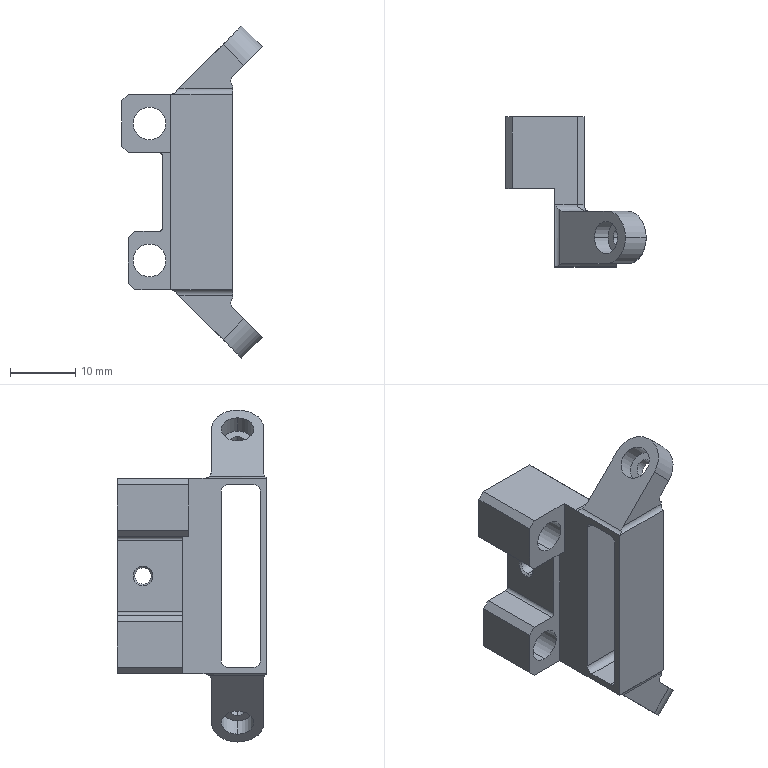NC program | NX | posted with a generic post | part box 21.534 x 23 x 50.912 mm
Lines 1 to 848 of 6474:
N10 G17 G21 G94 G90
(FLOOR_FACING , TOOL : D8开粗)
N12 T01 M6
N14 G54
N16 G17 G0 G90 X35. Y-12.5 B0. C0. S1061 M3
N18 G43 Z53. H1
N20 Z3.1
N22 G94 G1 Z0.1 F250.
N24 X34.
N26 G3 X32. Y-10.5 R2.
N28 G1 X-32.
N30 Y-5.55
N32 X32.
N34 Y-0.6
N36 X-32.
N38 Y4.35
N40 X32.
N42 Y9.3
N44 X-32.
N46 G3 X-34. Y7.3 R2.
N48 G1 X-35.
N50 Z3.1
N52 G0 Z53.
(ADAPTIVE_MILLING , TOOL : D8开粗)
N54 X37.12 Y1.02
N56 Z50.15
N58 Z-8.75
N60 G1 X36.97 Y1.008 Z-9.687
N62 X36.821 Y0.996 Z-10.058
N64 X36.671 Y0.985 Z-10.33
N66 X36.522 Y0.973 Z-10.55
N68 X36.372 Y0.961 Z-10.734
N70 X36.223 Y0.949 Z-10.892
N72 X36.073 Y0.938 Z-11.03
N74 X35.924 Y0.926 Z-11.15
N76 X35.774 Y0.914 Z-11.255
N78 X35.625 Y0.903 Z-11.348
N80 X35.475 Y0.891 Z-11.429
N82 X35.325 Y0.879 Z-11.5
N84 X35.176 Y0.867 Z-11.56
N86 X35.026 Y0.856 Z-11.612
N88 X34.877 Y0.844 Z-11.655
N90 X34.727 Y0.832 Z-11.689
N92 X34.578 Y0.821 Z-11.716
N94 X34.428 Y0.809 Z-11.735
N96 X34.279 Y0.797 Z-11.746
N98 X34.129 Y0.785 Z-11.75
N100 X32.743 Y0.677
N102 G3 X32.087 Y0.238 R0.809
N104 X31.465 Y-2.339 R7.41
N106 X31.241 Y-8.744 R74.09
N108 G2 X31.185 Y-10.771 R16.326
N110 X29.104 Y-13.79 R4.795
N112 X25.181 Y-15.269 R9.684
N114 X19.381 Y-15.687 R39.045
N116 X9.602 Y-15.727 R696.065
N118 G1 X-25.793 Y-15.726
N120 G2 X-28.856 Y-14.155 R4.335
N122 X-30.639 Y-10.333 R8.413
N124 X-31.16 Y-4.966 R29.566
N126 X-31.212 Y10.529 R651.721
N128 X-29.4 Y13.594 R4.522
N130 X-25.566 Y15.208 R8.891
N132 X-20.012 Y15.675 R33.85
N134 X-9.272 Y15.728 R699.457
N136 G1 X25.841 Y15.725
N138 G2 X29.013 Y14.001 R4.415
N140 X30.693 Y10.133 R8.704
N142 X31.174 Y4.52 R33.321
N144 X30.916 Y-0.16 R24.978
N146 G3 X30.457 Y-8.115 R78.765
N148 G2 X27.712 Y-12.707 R6.046
N150 X23.193 Y-14.403 R11.375
N152 X16.917 Y-14.876 R41.945
N154 X4.087 Y-14.924 R878.762
N156 G1 X-0.233 Y-14.927
N158 X-23.406 Y-14.925
N160 G2 X-28.115 Y-12.318 R5.94
N162 X-29.863 Y-7.885 R10.966
N164 X-30.367 Y-1.792 R38.718
N166 X-30.407 Y8.287 R314.055
N168 X-27.773 Y12.664 R5.962
N170 X-23.265 Y14.392 R11.16
N172 X-17.11 Y14.874 R40.717
N174 X-6.55 Y14.927 R694.796
N176 G1 X23.44 Y14.925
N178 G2 X28.138 Y12.306 R5.921
N180 X29.884 Y7.805 R11.093
N182 X30.132 Y0.751 R26.451
N184 G3 X29.694 Y-6.493 R229.838
N186 G2 X26.24 Y-11.917 R7.083
N188 X21.328 Y-13.608 R13.219
N190 X16.67 Y-14.034 R47.013
N192 G3 X16.304 Y-14.218 R1.352
N194 G2 X14.032 Y-14.914 R4.432
N196 G3 X16.495 Y-14.066 R4.204
N198 G2 X18.579 Y-13.556 R8.285
N200 G3 X23.029 Y-12.653 R30.768
N202 X27.011 Y-10.273 R8.809
N204 X28.853 Y-6.398 R8.238
N206 X29.458 Y-1.579 R39.94
N208 X29.703 Y4.352 R45.756
N210 X28.814 Y9.475 R17.252
N212 X26.213 Y12.898 R6.567
N214 X22.308 Y14.169 R9.553
N216 X16.977 Y14.431 R46.853
N218 G1 X10.977 Y14.447
N220 X-10.063 Y14.445
N222 G3 X-19.6 Y14.277 R171.741
N224 X-24.618 Y13.448 R20.333
N226 X-27.927 Y11.363 R7.158
N228 X-29.544 Y7.594 R8.07
N230 X-29.906 Y2.453 R31.43
N232 X-29.622 Y-5.818 R72.414
N234 X-28.473 Y-10.271 R13.972
N236 X-24.269 Y-13.763 R6.431
N238 X-19.941 Y-14.362 R18.143
N240 X-9.142 Y-14.447 R324.916
N242 G1 X3.318 Y-14.445
N244 G2 X5.099 Y-14.465 R18.722
N246 G3 X6.999 Y-14.917 R4.927
N248 G2 X4.896 Y-14.335 R4.42
N250 G3 X1.969 Y-13.818 R10.606
N252 X-5.593 Y-13.663 R111.649
N254 G2 X-7.001 Y-13.917 R4.701
N256 G1 X-14.001
N258 G3 X-19.53 Y-13.568 R111.918
N260 G2 X-23.365 Y-12.927 R14.578
N262 X-27.379 Y-9.236 R7.304
N264 X-28.751 Y-4.343 R14.883
N266 X-28.898 Y5.599 R49.455
N268 X-27.819 Y9.127 R8.415
N270 X-24.01 Y12.22 R7.937
N272 X-18.872 Y13.364 R17.751
N274 X-10.479 Y13.637 R99.34
N276 G1 X-3.639 Y13.647
N278 X12.961 Y13.645
N280 G2 X20.337 Y13.487 R104.564
N282 X23.841 Y12.733 R10.991
N284 X27.503 Y8.968 R7.427
N286 X28.724 Y3.434 R14.681
N288 X28.181 Y-5.054 R41.969
N290 X23.713 Y-10.998 R8.122
N292 X19.632 Y-12.405 R18.072
N294 G3 X17.794 Y-12.905 R28.33
N296 G1 X17.601 Y-13.035
N298 G2 X16.424 Y-14.12 R9.618
N300 G3 X17.729 Y-12.908 R10.801
N302 G2 X19.648 Y-12.042 R7.886
N304 G3 X23.329 Y-10.5 R20.797
N306 X27.297 Y-5.403 R8.58
N308 X28.174 Y0.275 R23.637
N310 X27.748 Y6.299 R20.911
N312 X25.598 Y10.397 R8.618
N314 X21.373 Y12.578 R8.611
N316 X16.129 Y13.11 R27.016
N318 X7.189 Y13.166 R509.255
N320 G1 X-7.191 Y13.164
N322 G3 X-17.268 Y12.979 R172.599
N324 X-22.634 Y12.06 R21.257
N326 X-26.611 Y9.275 R7.836
N328 X-28.256 Y4.875 R10.084
N330 X-28.016 Y-5.402 R33.893
N332 X-26.27 Y-9.642 R10.515
N334 X-22.087 Y-12.408 R7.883
N336 X-17.533 Y-13.134 R22.262
N338 G2 X-16.247 Y-13.262 R10.665
N340 G3 X-14.811 Y-13.837 R5.43
N342 G2 X-16.467 Y-13.123 R5.156
N344 G3 X-18.577 Y-12.452 R10.199
N346 G2 X-22.125 Y-11.356 R18.375
N348 X-26.286 Y-6.887 R8.47
N350 X-27.527 Y-1.287 R17.657
N352 X-27.278 Y4.809 R22.462
N354 X-22.759 Y10.591 R7.975
N356 X-17.686 Y11.966 R16.095
N358 X-10.019 Y12.342 R70.153
N360 G1 X-0.659 Y12.366
N362 G2 X15.52 Y12.307 R846.975
N364 X20.523 Y11.773 R24.745
N366 X26.155 Y6.979 R7.927
N368 X27.214 Y1.474 R14.843
N370 X26.52 Y-4.461 R19.027
N372 X22.391 Y-9.613 R9.101
N374 X19.109 Y-11.314 R44.702
N376 G3 X18.654 Y-11.692 R1.083
N378 G2 X17.679 Y-12.956 R4.45
N380 G3 X18.741 Y-11.535 R4.714
N382 G2 X20.145 Y-10.454 R6.268
N384 G3 X23.2 Y-8.283 R19.8
N386 X26.209 Y-2.814 R10.327
N388 X26.114 Y5.091 R16.811
N390 X20.517 Y10.939 R8.188
N392 X15.556 Y11.751 R19.568
N394 X7.758 Y11.884 R156.986
N396 G1 X-2.002 Y11.886
N398 G3 X-14. Y11.752 R297.339
N400 X-19.937 Y10.971 R28.228
N402 X-24.242 Y8.672 R9.651
N404 X-26.636 Y4.111 R9.
N406 X-26.196 Y-5.321 R19.302
N408 X-21.051 Y-10.962 R8.843
N410 X-17.656 Y-12.191 R62.447
N412 G2 X-16.935 Y-12.701 R1.456
N414 G1 X-16.307 Y-13.217
N416 G2 X-17.604 Y-12.044 R13.06
N418 G3 X-19.864 Y-10.72 R15.94
N420 G2 X-23.859 Y-7.319 R10.597
N422 X-25.877 Y-1.593 R12.958
N424 X-25.487 Y4.231 R13.95
N426 X-20.996 Y9.257 R8.336
N428 X-15.742 Y10.672 R16.815
N430 X-8.315 Y11.054 R69.393
N432 X5.285 Y11.085 R895.884
N434 X14.882 Y10.948 R185.888
N436 X19.659 Y10.137 R18.007
N438 X24.828 Y4.896 R8.289
N440 X24.713 Y-3.985 R13.021
N442 X21.544 Y-8.176 R10.874
N444 G3 X19.284 Y-10.072 R56.957
N446 X19.078 Y-10.499 R1.13
N448 X19.344 Y-11.173 R0.802
N450 X19.928 Y-11.376 Z-11.71 R0.849
N452 G1 X20.866 Y-11.405 Z-11.65
N454 X21.18 Y-11.411 F2500.
N456 X21.493 Y-11.434
N458 G2 X22.14 Y-12.268 R0.8
N460 G1 X22.108 Y-12.629
N462 G2 X21.129 Y-13.229 R0.8
N464 G1 X20.207 Y-12.992
N466 X19.678 Y-12.86 Z-11.685 F250.
N468 X19.152 Y-12.716 Z-11.719
N470 G2 X18.77 Y-12.437 Z-11.75 R0.803
N472 X18.71 Y-11.587 R0.801
N474 G3 X19.097 Y-10.339 R3.698
N476 G2 X20.019 Y-9.081 R3.844
N478 G3 X22.492 Y-6.448 R31.236
N480 X24.787 Y2.037 R11.638
N482 X22.508 Y7.292 R9.028
N484 X17.894 Y9.854 R9.45
N486 X12.544 Y10.512 R25.892
N488 X0.545 Y10.605 R372.56
N490 X-11.754 Y10.476 R327.243
N492 X-17.878 Y9.721 R31.
N494 X-22.412 Y7.466 R10.532
N496 X-25.135 Y2.287 R8.876
N498 X-23.934 Y-5.827 R12.942
N500 X-20.349 Y-9.652 R10.833
N502 G2 X-18.628 Y-10.811 R38.625
N504 G3 X-17.511 Y-12.125 R8.523
N506 G2 X-18.728 Y-10.58 R5.415
N508 G3 X-20.411 Y-8.788 R17.982
N510 G2 X-24.138 Y1.3 R12.178
N512 X-19.591 Y7.765 R8.256
N514 X-14.44 Y9.303 R15.958
N516 X-7.019 Y9.762 R60.13
N518 X11.28 Y9.733 R602.927
N520 X16.759 Y9.139 R27.875
N522 X21.279 Y6.681 R8.907
N524 X23.64 Y0.225 R9.126
N526 X21.384 Y-6.012 R10.678
N528 G3 X19.393 Y-8.599 R105.948
N530 X19.15 Y-9.175 R1.215
N532 G2 X19.085 Y-10.424 R8.334
N534 G3 X19.153 Y-8.995 R9.581
N536 G2 X19.978 Y-7.313 R5.486
N538 G3 X21.97 Y-3.945 R24.564
N540 X22.367 Y3.36 R9.691
N542 X17.757 Y7.991 R8.057
N544 X12.736 Y9.092 R16.908
N546 X4.581 Y9.32 R102.883
N548 X-9.158 Y9.218 R435.23
N550 X-15.593 Y8.536 R36.388
N552 X-20.188 Y6.562 R11.757
N554 X-23.419 Y0.22 R8.31
N556 X-20.828 Y-7.342 R11.195
N558 G1 X-19.172 Y-9.335
N560 X-19.073 Y-9.553
N562 G2 X-19.351 Y-10.237 R0.802
N564 X-19.989 Y-10.422 Z-11.707 R0.841
N566 G1 X-20.875 Y-10.371 Z-11.65
N568 X-21.159 Y-10.352 F2500.
N570 X-21.443 Y-10.35
N572 G3 X-22.135 Y-11.321 R0.8
N574 G1 X-22.089 Y-11.529
N576 X-22.03 Y-11.734
N578 G3 X-21.143 Y-12.215 R0.8
N580 G1 X-20.186 Y-12.035
N582 X-19.642 Y-11.937 Z-11.685 F250.
N584 X-19.101 Y-11.823 Z-11.72
N586 G3 X-18.728 Y-11.555 Z-11.75 R0.832
N588 X-18.655 Y-10.689 R0.801
N590 G2 X-19.116 Y-9.278 R3.972
N592 G3 X-19.907 Y-7.64 R8.536
N594 G2 X-21.801 Y-3.654 R18.639
N596 X-21.825 Y2.011 R9.094
N598 X-17.953 Y6.378 R8.098
N600 X-12.636 Y8.008 R15.833
N602 X-5.036 Y8.481 R60.813
N604 X9.783 Y8.433 R371.174
N606 X15.251 Y7.762 R25.753
N608 X19.652 Y5.203 R8.615
N610 X21.344 Y-1.739 R7.995
N612 X19.87 Y-5.598 R15.266
N614 G3 X19.168 Y-7.098 R13.871
N616 X19.15 Y-9.077 R30.242
N618 G2 X19.173 Y-6.872 R30.099
N620 X19.927 Y-4.544 R15.286
N622 G3 X20.8 Y-0.216 R11.824
N624 X16.599 Y6.369 R7.406
N626 X11.707 Y7.715 R14.412
N628 X4.637 Y8.028 R66.907
N630 X-8.201 Y7.895 R274.818
N632 X-14.437 Y7.082 R30.758
N634 X-18.914 Y4.825 R10.629
N636 X-21.363 Y-1.693 R7.733
N638 X-20.027 Y-6.151 R12.999
N640 G2 X-19.166 Y-8.067 R20.478
N642 G3 X-19.085 Y-9.423 R16.666
N644 G2 X-19.162 Y-7.572 R15.691
N646 G3 X-19.844 Y-4.784 R23.582
N648 G2 X-20.199 Y-0.45 R10.636
N650 X-16.663 Y4.748 R7.537
N652 X-11.608 Y6.584 R14.005
N654 X-4.619 Y7.168 R46.823
N656 X8.698 Y7.11 R211.754
N658 X13.906 Y6.321 R21.683
N660 X17.945 Y3.64 R7.779
N662 X19.331 Y-1.506 R7.629
N664 X19.15 Y-3.007 R38.763
N666 G1 Y-7.147
N668 Y0.233
N670 G3 X17.935 Y3.167 R4.319
N672 X16.307 Y4.683 R14.745
N674 X12.854 Y5.969 R12.331
N676 X6.604 Y6.673 R32.118
N678 X-7.192 Y6.561 R177.858
N680 X-13.051 Y5.661 R26.641
N682 G2 X-14.808 Y5.304 R5.067
N684 G3 X-16.934 Y4.168 R4.465
N686 X-18.45 Y2.54 R14.745
N688 X-19.497 Y-1.029 R7.838
N690 X-19.51 Y-5.027 R71.203
N692 G2 X-19.15 Y-6.133 R6.719
N694 G1 Y-7.753
N696 Y0.234
N698 G2 X-17.934 Y3.168 R4.32
N700 X-16.304 Y4.684 R14.694
N702 X-13.968 Y5.383 R4.458
N704 G3 X-9.622 Y5.572 R35.322
N706 G2 X7.647 Y5.788 R148.811
N708 X11.183 Y5.383 R34.41
N710 G1 X14.001
N712 G2 X15.589 Y5.067 R4.814
N714 G3 X14.001 Y5.383 R4.813
N716 G2 X1.185 Y5.445 R937.203
N718 X-12.241 Y5.383 R784.161
N720 G1 X6.839
N722 G3 X7.508 Y5.745 R0.801
N724 G1 X7.694 Y6.029
N726 X8.554 Y7.345 Z-11.65
N728 G2 X8.848 Y7.715 R1.39 F2500.
N730 X9.339 Y7.884 R0.808
N732 G1 X14.742
N734 G2 X16.154 Y7.552 R3.292
N736 G1 X16.584 Y7.32
N738 X17.179 Y6.951
N740 X17.769 Y6.575
N742 G2 X19.613 Y4.893 R9.035
N744 X20.378 Y3.899 R9.537
N746 X21.375 Y1.05 R6.429
N748 X21.639 Y-2.864 R62.209
N750 G1 X21.721 Y-5.108
N752 X21.787 Y-7.352
N754 G2 X21.477 Y-10.687 R17.537
N756 G1 X21.355 Y-11.328
N758 X21.222 Y-11.968
N760 G2 X19.345 Y-14.932 R5.689
N762 G1 X18.643 Y-15.522
N764 X17.929 Y-16.099
N766 G2 X15.633 Y-17.063 R5.421
N768 X12.712 Y-17.333 R20.149
N770 G1 X6.769 Y-17.444
N772 G2 X5.968 Y-16.809 R0.806
N774 G1 X5.522 Y-15.302 Z-11.75 F250.
N776 X5.441 Y-15.019
N778 X5.345 Y-14.741
N780 G3 X5.001 Y-14.381 R0.81
N782 G1 X4.179 Y-13.889
N784 G3 X1.165 Y-13.157 R9.756
N786 X-4.134 Y-12.913 R46.955
N788 X-4.696 Y-13.218 R1.123
N790 G2 X-5.7 Y-13.688 R4.155
N792 G3 X-4.374 Y-12.958 R3.677
N794 G2 X-2.494 Y-12.614 R5.274
N796 X3.078 Y-13.124 R18.173
N798 X4.065 Y-13.701 R1.671
N800 G1 X4.622 Y-14.158
N802 G2 X3.49 Y-13.141 R12.628
N804 G3 X1.113 Y-12.221 R5.917
N806 X-3.263 Y-12.094 R12.119
N808 X-3.652 Y-12.288 R1.303
N810 G2 X-4.437 Y-13.006 R8.108
N812 G3 X-3.522 Y-12.163 R9.759
N814 G2 X-1.685 Y-11.687 R4.118
N816 X2.697 Y-12.361 R9.416
N818 X3.065 Y-12.701 R1.339
N820 G1 X3.617 Y-13.252
N822 G2 X2.648 Y-12.218 R17.979
N824 G3 X0.162 Y-11.228 R5.122
N826 X-2.643 Y-11.332 R6.396
N828 X-3.066 Y-11.702 R1.145
N830 G1 X-3.575 Y-12.211
N832 G3 X-2.819 Y-11.401 R9.091
N834 G2 X-1.001 Y-10.885 R3.302
N836 X2.214 Y-11.62 R5.863
N838 X2.549 Y-12.071 R1.25
N840 G1 X2.777 Y-12.35
N842 G2 X2.323 Y-11.648 R2.718
N844 G3 X0.623 Y-10.627 R3.169
N846 X-2.157 Y-10.656 R4.441
N848 X-2.466 Y-10.935 R1.443
N850 X-2.505 Y-11.805 R0.881
N852 X-1.819 Y-12.283 Z-11.695 R0.912
N854 G1 X-1.131 Y-12.421 Z-11.65
N856 X0.699 Y-12.79 F2500.
N858 X1.097 Y-12.872 Z-11.676 F250.
N860 X1.498 Y-12.941 Z-11.702
N862 G3 X2.181 Y-12.672 Z-11.75 R0.893
N864 X2.323 Y-11.648 R0.88
N866 X0.75 Y-10.304 R2.616
N868 X-1.85 Y-10.174 R3.81
N870 X-2.274 Y-10.54 R0.976
N872 G2 X-2.884 Y-11.477 R2.794
N874 G3 X-2.189 Y-10.382 R3.756
N876 G2 X-0.883 Y-9.84 R1.864
N878 X1.905 Y-10.758 R3.651
N880 X2.165 Y-11.354 R1.438
N882 G3 X1.704 Y-10.37 R2.089
N884 X-1.71 Y-9.697 R3.149
N886 X-2.091 Y-10.146 R0.954
N888 X-1.982 Y-10.912 R0.882
N890 X-1.401 Y-11.289 Z-11.705 R0.926
N892 G1 X-0.567 Y-11.506 Z-11.65
N894 X0.215 Y-11.711 F2500.
N896 X0.639 Y-11.825 Z-11.678 F250.
N898 X1.067 Y-11.922 Z-11.706
N900 G3 X1.713 Y-11.725 Z-11.75 R0.9
N902 X1.995 Y-10.791 R0.881
N904 X0.755 Y-9.416 R2.074
N906 X-1.581 Y-9.326 R2.757
N908 X-2.012 Y-9.827 R0.912
N910 G2 X-2.245 Y-10.483 R1.953
N912 G3 X-1.962 Y-9.654 R3.024
N914 G2 X-1.018 Y-9.021 R1.317
N916 X1.781 Y-9.995 R2.801
N918 X1.93 Y-10.575 R1.235
N920 G3 X1.149 Y-9.131 R1.617
N922 X-1.53 Y-8.916 R2.68
N924 X-1.906 Y-9.408 R0.924
N926 G1 X-2.009 Y-9.815
N928 G2 X-1.746 Y-9.057 R2.324
N930 X-0.998 Y-8.667 R0.967
N932 G1 X-0.638
N934 G3 X-1.603 Y-8.886 R1.364
N936 X-1.796 Y-9.141 R2.258
N938 G1 X-1.712 Y-9.005
N940 X-1.603 Y-8.886
N942 G2 X-1.199 Y-8.691 R0.976
N944 X0.56 Y-8.714 R7.837
N946 X1.796 Y-9.612 R1.877
N948 X1.883 Y-10.107 R2.226
N950 G3 X1.783 Y-9.406 R2.396
N952 X0.861 Y-8.667 R1.196
N954 G1 X0.201
N956 X1.058 Y-8.677
N958 G2 X1.85 Y-9.759 R0.991
N960 G3 X0.99 Y-8.67 R0.936
N962 X0.153 Y-9.278 R0.808
N964 G1 X-0.193 Y-10.646
N966 X-0.23 Y-10.792 Z-11.746
N968 X-0.266 Y-10.937 Z-11.735
N970 X-0.303 Y-11.082 Z-11.716
N972 X-0.34 Y-11.228 Z-11.689
N974 X-0.377 Y-11.373 Z-11.655
N976 X-0.414 Y-11.519 Z-11.612
N978 X-0.45 Y-11.664 Z-11.56
N980 X-0.487 Y-11.809 Z-11.5
N982 X-0.524 Y-11.955 Z-11.429
N984 X-0.561 Y-12.1 Z-11.348
N986 X-0.598 Y-12.246 Z-11.255
N988 X-0.634 Y-12.391 Z-11.15
N990 X-0.671 Y-12.537 Z-11.03
N992 X-0.708 Y-12.682 Z-10.892
N994 X-0.745 Y-12.827 Z-10.734
N996 X-0.781 Y-12.973 Z-10.55
N998 X-0.818 Y-13.118 Z-10.33
N1000 X-0.855 Y-13.264 Z-10.058
N1002 X-0.892 Y-13.409 Z-9.687
N1004 X-0.929 Y-13.554 Z-8.75
N1006 G0 Z50.15
N1008 X37.035 Y9.181
N1010 Z-20.5
N1012 G1 X36.885 Y9.173 Z-21.437
N1014 X36.736 Y9.166 Z-21.808
N1016 X36.586 Y9.158 Z-22.08
N1018 X36.436 Y9.15 Z-22.3
N1020 X36.286 Y9.142 Z-22.484
N1022 X36.136 Y9.134 Z-22.642
N1024 X35.987 Y9.127 Z-22.78
N1026 X35.837 Y9.119 Z-22.9
N1028 X35.687 Y9.111 Z-23.005
N1030 X35.537 Y9.103 Z-23.098
N1032 X35.387 Y9.096 Z-23.179
N1034 X35.238 Y9.088 Z-23.25
N1036 X35.088 Y9.08 Z-23.31
N1038 X34.938 Y9.072 Z-23.362
N1040 X34.788 Y9.065 Z-23.405
N1042 X34.638 Y9.057 Z-23.439
N1044 X34.489 Y9.049 Z-23.466
N1046 X34.339 Y9.041 Z-23.485
N1048 X34.189 Y9.033 Z-23.496
N1050 X34.039 Y9.026 Z-23.5
N1052 X32.727 Y8.958
N1054 G3 X32.035 Y8.489 R0.809
N1056 X31.424 Y5.83 R7.923
N1058 X31.212 Y-0.254 R75.67
N1060 G1 X31.183 Y-10.495
N1062 G2 X29.335 Y-13.563 R4.577
N1064 X25.507 Y-15.171 R9.007
N1066 X20.014 Y-15.643 R33.134
N1068 X9.934 Y-15.698 R678.761
N1070 G1 X-25.763 Y-15.696
N1072 G2 X-28.905 Y-14.036 R4.375
N1074 X-30.636 Y-10.183 R8.625
N1076 X-31.139 Y-4.632 R31.583
N1078 X-31.184 Y10.491 R743.333
N1080 X-29.378 Y13.56 R4.516
N1082 X-25.486 Y15.188 R8.921
N1084 X-19.991 Y15.644 R34.222
N1086 X-9.371 Y15.698 R694.319
N1088 G1 X25.811 Y15.695
N1090 G2 X28.945 Y14.018 R4.391
N1092 X30.543 Y9.827 R7.236
N1094 X30.528 Y5.006 R44.553
N1096 G3 X30.391 Y-8.036 R454.834
N1098 G2 X27.739 Y-12.62 R5.976
N1100 X23.352 Y-14.335 R11.03
N1102 X17.439 Y-14.834 R37.763
N1104 G1 X14.383 Y-14.879
N1106 X13.999 Y-14.917
N1108 X1.762 Y-14.899
N1110 X-23.256 Y-14.898
N1112 G2 X-28.046 Y-12.344 R5.919
N1114 X-29.833 Y-7.86 R10.892
N1116 X-30.337 Y-1.828 R38.462
N1118 X-30.376 Y8.271 R273.53
N1120 X-27.671 Y12.684 R5.997
N1122 X-24.895 Y13.98 R10.289
N1124 G3 X-24.473 Y14.285 R7.331
N1126 G1 X-23.628 Y14.689
N1128 X-22.713 Y14.892
N1130 G3 X-12.059 Y14.896 R826.111
N1132 G1 X23.291 Y14.897
N1134 G2 X28.264 Y11.823 R5.624
N1136 X29.18 Y9.354 R10.099
N1138 G1 X29.373 Y8.953
N1140 G2 X29.64 Y6.787 R7.278
N1142 X29.608 Y-2.765 R484.114
N1144 X29.557 Y-6.598 R62.516
N1146 X26.144 Y-11.896 R6.983
N1148 X21.295 Y-13.573 R13.105
N1150 X16.757 Y-13.991 R41.212
N1152 G3 X16.304 Y-14.218 R1.062
N1154 G2 X14.808 Y-14.837 R4.811
N1156 G1 X14.33 Y-14.884
N1158 G3 X16.541 Y-14.029 R3.931
N1160 G2 X18.731 Y-13.499 R8.934
N1162 G3 X23.234 Y-12.533 R27.296
N1164 X27.114 Y-10.012 R8.353
N1166 X28.746 Y-6.121 R8.302
N1168 X29.114 Y-0.979 R35.495
N1170 X29.178 Y5.74 R592.028
N1172 G2 X29.371 Y6.212 R3.245
N1174 G1 X29.578 Y7.117
N1176 X29.579 Y8.047
N1178 X29.578 Y7.117
N1180 X29.371 Y6.212
N1182 G3 X28.637 Y3.66 R6.596
N1184 X28.277 Y-2.181 R87.754
N1186 G2 X27.71 Y-6.212 R17.73
N1188 X23.791 Y-10.867 R7.867
N1190 X19.732 Y-12.336 R16.968
N1192 G3 X17.837 Y-12.86 R28.301
N1194 G1 X17.65 Y-12.986
N1196 G2 X16.47 Y-14.082 R9.781
N1198 G3 X17.778 Y-12.86 R11.315
N1200 G2 X19.625 Y-12.009 R7.792
N1202 G3 X23.317 Y-10.414 R20.246
N1204 X27.123 Y-5.28 R8.374
N1206 X27.809 Y-0.719 R23.368
N1208 G2 X28.249 Y3.886 R50.21
N1210 X28.509 Y4.8 R2.636
N1212 G3 X29.072 Y5.591 R3.313
N1214 G2 X28.509 Y4.8 R3.313
N1216 G3 X27.673 Y3.004 R4.261
N1218 X27.004 Y-1.181 R36.176
N1220 G2 X25.99 Y-5.428 R15.993
N1222 X22.076 Y-9.71 R9.291
N1224 X18.983 Y-11.338 R69.974
N1226 G3 X18.687 Y-11.63 R1.415
N1228 G2 X17.722 Y-12.914 R4.424
N1230 G3 X18.774 Y-11.473 R4.737
N1232 G2 X20.115 Y-10.414 R6.311
N1234 G3 X23.149 Y-8.187 R19.616
N1236 X25.956 Y-3.229 R10.471
N1238 X26.846 Y1.256 R55.683
N1240 G2 X27.578 Y3.807 R10.802
N1242 X28.387 Y4.647 R9.294
N1244 G3 X27.206 Y3.417 R12.494
N1246 X26.181 Y0.881 R8.666
N1248 G2 X25.084 Y-3.051 R51.405
N1250 X21.336 Y-8.279 R11.817
N1252 G3 X19.276 Y-10.041 R38.663
N1254 X19.07 Y-10.578 R0.974
N1256 G2 X18.72 Y-11.568 R4.277
N1258 G3 X19.102 Y-10.29 R3.713
N1260 G2 X20.009 Y-9.033 R3.971
N1262 G3 X22.522 Y-6.332 R34.824
N1264 X24.952 Y-1.474 R15.13
N1266 G2 X26.119 Y2.077 R48.333
N1268 X26.441 Y2.7 R3.24
N1270 G1 X27.374 Y3.634
N1272 G3 X25.904 Y2.129 R24.3
N1274 X24.635 Y-0.361 R11.947
N1276 G2 X22.419 Y-4.767 R22.812
N1278 X19.876 Y-7.952 R45.457
N1280 G3 X19.181 Y-8.999 R4.044
N1282 X19.15 Y-9.768 R3.591
N1284 G1 X19.091 Y-10.365
N1286 G3 X19.153 Y-8.996 R9.469
N1288 G2 X20.071 Y-7.228 R5.374
N1290 G3 X22.573 Y-3.461 R39.167
N1292 X24.495 Y0.501 R88.411
N1294 G2 X24.828 Y1.088 R11.169
N1296 G1 X26.101 Y2.361
N1298 G3 X24.073 Y0.305 R77.035
N1300 X22.196 Y-2.578 R29.762
N1302 G2 X19.678 Y-6.425 R445.696
N1304 G3 X19.156 Y-7.484 R3.556
N1306 G1 X19.15 Y-9.103
N1308 X19.152 Y-7.363
N1310 G2 X19.99 Y-5.333 R6.439
N1312 X22.446 Y-1.295 R181.538
N1314 G1 X24.27 Y0.53
N1316 G3 X21.009 Y-2.754 R457.095
N1318 X19.177 Y-5.583 R11.439
N1320 G1 X19.15 Y-5.75
N1322 Y-7.43
N1324 X19.151 Y-5.57
N1326 G2 X19.797 Y-3.943 R4.399
N1328 G1 X21.197 Y-2.543
N1330 G3 X19.335 Y-4.429 R206.58
N1332 X19.15 Y-5.004 R1.101
N1334 G1 Y-5.664
N1336 G3 X19.731 Y-6.434 R0.8
N1338 X20.481 Y-6.268 Z-23.449 R0.831
N1340 G1 X21.107 Y-5.816 Z-23.4
N1342 X22.469 Y-4.832 F2500.
N1344 X22.566 Y-4.749
N1346 X30.405 Y3.09
N1348 G3 X31.919 Y5.933 R5.523
N1350 G1 X32.243 Y7.586
N1352 G3 X31.622 Y8.523 R0.8
N1354 G1 X31.495 Y8.549
N1356 X29.957 Y8.872 Z-23.5 F250.
N1358 G2 X29.509 Y9.003 R1.513
N1360 X29.18 Y9.354 R0.811
N1362 G3 X27.206 Y12.188 R10.52
N1364 X25.633 Y13.278 R8.593
N1366 X24.473 Y14.285 R8.109
N1368 G1 X23.628 Y14.689
N1370 X22.713 Y14.892
N1372 X21.777 Y14.886
N1374 G2 X18.248 Y14.481 R15.299
N1376 X10.269 Y14.418 R360.661
N1378 G1 X-11.771 Y14.416
N1380 X-20.259 Y14.413
N1382 G2 X-20.866 Y14.67 R2.509
N1384 G1 X-21.777 Y14.886
N1386 X-20.866 Y14.67
N1388 G3 X-18.288 Y13.886 R6.267
N1390 X-12.088 Y13.633 R59.747
N1392 G1 X-5.268 Y13.618
N1394 X12.363 Y13.62
N1396 G3 X19.248 Y13.785 R88.659
N1398 X19.636 Y13.936 R1.448
N1400 G1 X20.026 Y14.255
N1402 X20.866 Y14.67
N1404 X21.216 Y14.753
N1406 X20.866 Y14.67
N1408 X20.026 Y14.255
N1410 G2 X19.347 Y13.755 R2.787
N1412 X16.718 Y13.288 R9.373
N1414 X8.588 Y13.139 R133.607
N1416 G1 X-5.509 Y13.138
N1418 G2 X-15.9 Y13.251 R251.139
N1420 X-19.286 Y13.694 R15.199
N1422 X-20.026 Y14.255 R4.629
N1424 G1 X-20.134 Y14.309
N1426 G2 X-19.255 Y13.623 R5.585
N1428 G3 X-17.087 Y12.829 R5.402
N1430 X-11.85 Y12.4 R33.657
N1432 X-1.008 Y12.339 R633.422
N1434 X14.079 Y12.396 R752.114
N1436 X18.103 Y12.773 R22.282
N1438 X18.642 Y13.004 R1.224
N1440 G2 X19.577 Y13.888 R9.689
N1442 G3 X18.512 Y12.878 R12.084
N1444 G2 X16.543 Y12.233 R5.247
N1446 X11.234 Y11.892 R38.371
N1448 X-2.869 Y11.859 R921.682
N1450 X-13.372 Y11.995 R233.773
N1452 X-17.736 Y12.597 R19.721
N1454 X-18.605 Y12.967 R2.735
N1456 G1 X-19.3 Y13.662
N1458 G3 X-18.166 Y12.567 R13.625
N1460 X-15.485 Y11.607 R7.108
N1462 X-9.919 Y11.136 R36.829
N1464 X11.978 Y11.125 R717.047
N1466 X16.724 Y11.595 R24.92
N1468 X17.555 Y11.917 R1.944
N1470 G1 X18.574 Y12.935
N1472 X17.427 Y11.791
N1474 G2 X15.463 Y11.067 R5.203
N1476 X10.59 Y10.646 R30.422
N1478 X-10.073 Y10.674 R575.939
N1480 X-15.673 Y11.239 R31.684
N1482 X-17.5 Y11.869 R6.244
N1484 G1 X-18.352 Y12.714
N1486 G3 X-17.055 Y11.458 R15.921
N1488 X-14.392 Y10.442 R7.364
N1490 G1 X-14.077 Y10.383
N1492 X14.521 Y10.39
N1494 G3 X16.339 Y10.749 R6.191
N1496 G1 X16.491 Y10.853
N1498 X17.509 Y11.871
N1500 X16.361 Y10.728
N1502 G2 X15.569 Y10.383 R1.903
N1504 G1 X14.369
N1506 G3 X15.831 Y10.411 R10.355
N1508 X16.441 Y10.803 R1.231
N1510 G1 X19.298 Y13.66
N1512 X20.026 Y14.255
N1514 X20.866 Y14.67
N1516 X21.777 Y14.886
N1518 X22.713 Y14.892
N1520 X23.628 Y14.689
N1522 X24.473 Y14.285
N1524 G2 X25.613 Y13.295 R7.712
N1526 G1 X28.392 Y10.517
N1528 X28.97 Y9.791
N1530 G3 X29.333 Y9.533 R0.816
N1532 G1 X29.936 Y9.323
N1534 X31.42 Y8.804 Z-23.4
N1536 G2 X32.033 Y8.022 R0.821 F2500.
N1538 G1 X32.036 Y7.394
N1540 X32.023 Y6.766
N1542 G2 X31.539 Y5.209 R3.646
N1544 G1 X21.898 Y-11.342
N1546 G2 X18.861 Y-15.134 R16.516
N1548 G1 X18.349 Y-15.612
N1550 X17.827 Y-16.079
N1552 G2 X15.706 Y-17.139 R5.404
N1554 X12.956 Y-17.457 R10.982
N1556 G1 X9.5 Y-17.417
N1558 G2 X8.854 Y-17.077 R0.802
N1560 G1 X8.726 Y-16.894
N1562 X7.823 Y-15.607 Z-23.5 F250.
N1564 X7.663 Y-15.372
N1566 X7.487 Y-15.148
N1568 G3 X6.999 Y-14.917 R0.807
N1570 G2 X5.411 Y-14.6 R4.814
N1572 G3 X1.295 Y-14.178 R21.698
N1574 X-9.757 Y-14.099 R427.923
N1576 G2 X-21.816 Y-14.078 R835.009
N1578 X-27.382 Y-10.665 R6.963
N1580 X-29.068 Y-5.821 R13.058
N1582 X-29.541 Y0.577 R46.428
N1584 X-29.563 Y6.456 R114.145
N1586 G3 X-29.577 Y7.103 R1.681
N1588 G1 X-29.58 Y8.036
N1590 X-29.375 Y8.946
N1592 X-28.972 Y9.787
N1594 X-28.391 Y10.518
N1596 X-25.205 Y13.703
N1598 X-24.735 Y14.076
N1600 X-25.205 Y13.703
N1602 X-28.391 Y10.518
N1604 X-28.972 Y9.787
N1606 X-29.375 Y8.946
N1608 X-29.58 Y8.036
N1610 X-29.577 Y7.103
N1612 G2 X-29.154 Y3.448 R16.561
N1614 G3 X-28.836 Y-3.463 R123.887
N1616 X-27.711 Y-8.54 R17.518
N1618 X-24.37 Y-12.358 R7.315
N1620 X-20.267 Y-13.42 R11.19
N1622 X-15.592 Y-13.609 R65.291
N1624 X-14.001 Y-13.917 R5.398
N1626 G1 X-7.001
N1628 G2 X-0.158 Y-13.678 R49.356
N1630 X4.317 Y-13.997 R30.805
N1632 X4.693 Y-14.217 R1.356
N1634 G1 X5.411 Y-14.6
N1636 G2 X4.284 Y-13.9 R5.03
N1638 G3 X1.771 Y-13.186 R7.131
N1640 X-4.239 Y-12.974 R35.504
N1642 X-4.696 Y-13.218 R1.098
N1644 G2 X-6.192 Y-13.837 R4.811
N1646 G3 X-4.429 Y-13.005 R4.263
N1648 G2 X-2.226 Y-12.603 R6.341
N1650 X3.012 Y-13.052 R17.342
N1652 X4.065 Y-13.701 R1.768
N1654 G1 X4.436 Y-14.005
N1656 G2 X3.398 Y-13.054 R15.907
N1658 G3 X0.97 Y-12.162 R5.951
N1660 X-3.356 Y-12.131 R11.618
N1662 X-3.669 Y-12.305 R3.087
N1664 G2 X-4.484 Y-13.044 R8.053
N1666 G3 X-3.539 Y-12.18 R9.511
N1668 G2 X-1.514 Y-11.668 R4.426
N1670 X2.662 Y-12.318 R9.057
N1672 X3.065 Y-12.701 R1.402
N1674 G1 X3.532 Y-13.168
N1676 G2 X2.615 Y-12.178 R16.867
N1678 G3 X0.198 Y-11.216 R4.954
N1680 X-2.655 Y-11.336 R6.424
N1682 X-3.066 Y-11.702 R1.179
N1684 G1 X-3.618 Y-12.253
N1686 G3 X-2.824 Y-11.407 R8.996
N1688 G2 X-1.05 Y-10.878 R3.278